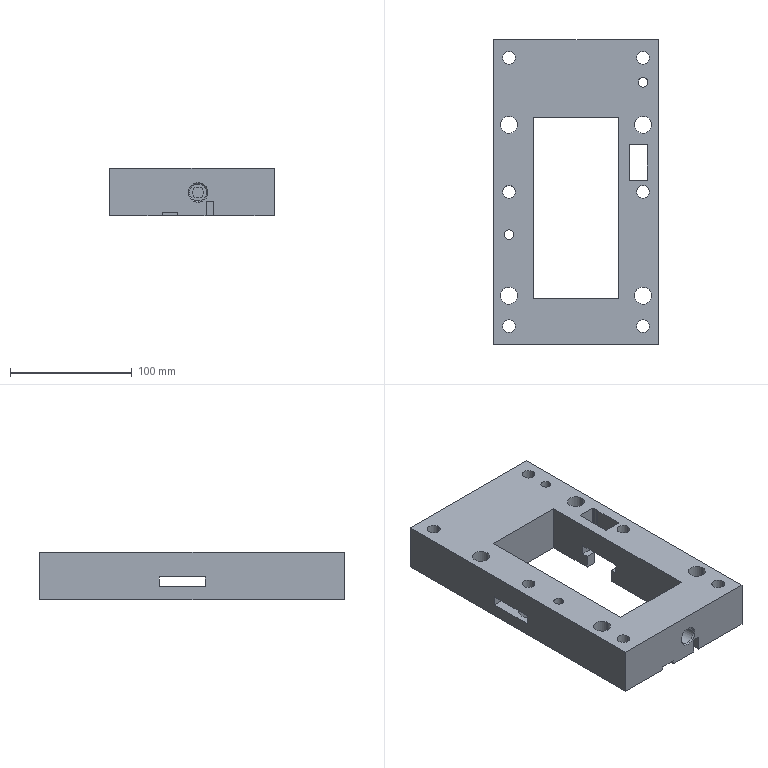Part | STEP file | KHUON BAO DUOI_2 | 1 solid | 93 faces | box 135 x 250 x 39.2 mm | volume 811850 mm3 | cylinder 47 | plane 44 | cone 2 | commonest cylinder face diameters 16 x13 10.5 x12 14 x10 8 x6 1 x4 9 x2